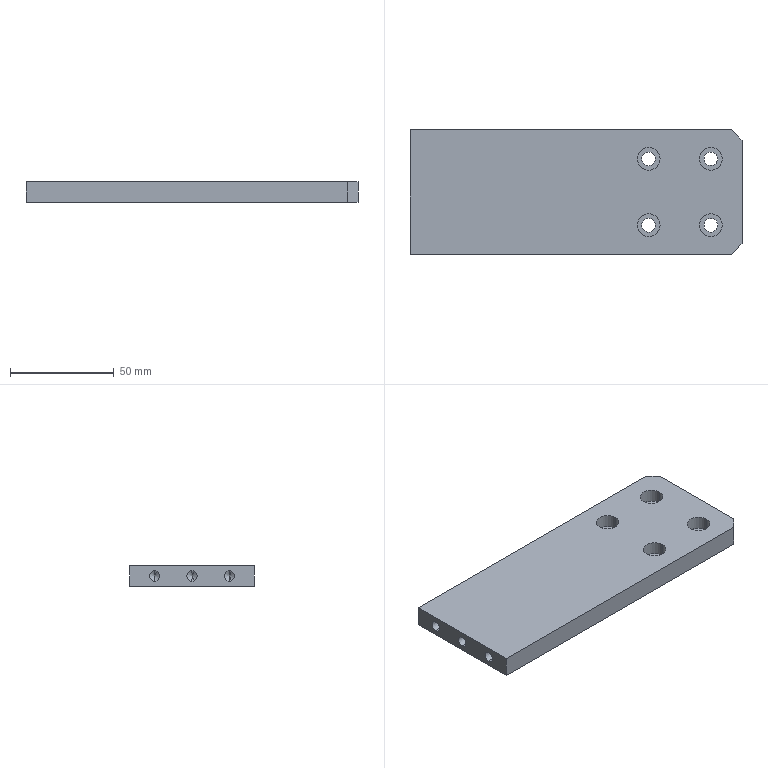Part | SolidWorks | features HoleWzd 2, Chamfer 1, Extrusion 1 | 1 solid | 40 faces | box 160 x 60 x 10 mm | volume 92147 mm3 | cylinder 22 | plane 12 | cone 6 | commonest cylinder face diameters 6.6 x8 11 x8 5 x6
STEP:
#1=CARTESIAN_POINT('',(-69.,18.,-2.5));
#2=VERTEX_POINT('',#1);
#3=CARTESIAN_POINT('',(-69.,18.,2.5));
#4=VERTEX_POINT('',#3);
#5=CARTESIAN_POINT('',(-69.,18.,0.));
#6=DIRECTION('',(-1.,0.,0.));
#7=DIRECTION('',(0.,0.,1.));
#8=AXIS2_PLACEMENT_3D('',#5,#6,#7);
#9=CIRCLE('',#8,2.5);
#10=EDGE_CURVE('',#2,#4,#9,.T.);
#11=ORIENTED_EDGE('',*,*,#10,.F.);
#12=CARTESIAN_POINT('',(-80.,18.,-2.5));
#13=VERTEX_POINT('',#12);
#14=CARTESIAN_POINT('',(-80.,18.,-2.5));
#15=DIRECTION('',(-1.,0.,0.));
#16=VECTOR('',#15,1000.);
#17=LINE('',#14,#16);
#18=EDGE_CURVE('',#2,#13,#17,.T.);
#19=ORIENTED_EDGE('',*,*,#18,.T.);
#20=CARTESIAN_POINT('',(-80.,18.,2.5));
#21=VERTEX_POINT('',#20);
#22=CARTESIAN_POINT('',(-80.,18.,0.));
#23=DIRECTION('',(-1.,0.,0.));
#24=DIRECTION('',(0.,0.,1.));
#25=AXIS2_PLACEMENT_3D('',#22,#23,#24);
#26=CIRCLE('',#25,2.5);
#27=EDGE_CURVE('',#13,#21,#26,.T.);
#28=ORIENTED_EDGE('',*,*,#27,.T.);
#29=CARTESIAN_POINT('',(-80.,18.,2.5));
#30=DIRECTION('',(-1.,0.,0.));
#31=VECTOR('',#30,1000.);
#32=LINE('',#29,#31);
#33=EDGE_CURVE('',#4,#21,#32,.T.);
#34=ORIENTED_EDGE('',*,*,#33,.F.);
#35=EDGE_LOOP('',(#11,#19,#28,#34));
#36=FACE_OUTER_BOUND('',#35,.T.);
#37=CARTESIAN_POINT('',(-80.,18.,0.));
#38=DIRECTION('',(-1.,0.,0.));
#39=DIRECTION('',(0.,0.,1.));
#40=AXIS2_PLACEMENT_3D('',#37,#38,#39);
#41=CYLINDRICAL_SURFACE('',#40,2.5);
#42=ADVANCED_FACE('',(#36),#41,.F.);
#43=CARTESIAN_POINT('',(-67.498,18.,0.));
#44=VERTEX_POINT('',#43);
#45=CARTESIAN_POINT('',(-69.,18.,2.5));
#46=DIRECTION('',(-0.515,0.,0.8572));
#47=VECTOR('',#46,1000.);
#48=LINE('',#45,#47);
#49=EDGE_CURVE('',#44,#4,#48,.T.);
#50=ORIENTED_EDGE('',*,*,#49,.F.);
#51=CARTESIAN_POINT('',(-69.,18.,-2.5));
#52=DIRECTION('',(-0.515,0.,-0.8572));
#53=VECTOR('',#52,1000.);
#54=LINE('',#51,#53);
#55=EDGE_CURVE('',#44,#2,#54,.T.);
#56=ORIENTED_EDGE('',*,*,#55,.T.);
#57=ORIENTED_EDGE('',*,*,#10,.T.);
#58=EDGE_LOOP('',(#50,#56,#57));
#59=FACE_OUTER_BOUND('',#58,.T.);
#60=CARTESIAN_POINT('',(-69.,18.,0.));
#61=DIRECTION('',(-1.,0.,0.));
#62=DIRECTION('',(0.,0.,1.));
#63=AXIS2_PLACEMENT_3D('',#60,#61,#62);
#64=CONICAL_SURFACE('',#63,2.5,1.03);
#65=ADVANCED_FACE('',(#59),#64,.F.);
#66=CARTESIAN_POINT('',(-69.,0.,-2.5));
#67=VERTEX_POINT('',#66);
#68=CARTESIAN_POINT('',(-69.,0.,2.5));
#69=VERTEX_POINT('',#68);
#70=CARTESIAN_POINT('',(-69.,0.,0.));
#71=DIRECTION('',(-1.,0.,0.));
#72=DIRECTION('',(0.,0.,1.));
#73=AXIS2_PLACEMENT_3D('',#70,#71,#72);
#74=CIRCLE('',#73,2.5);
#75=EDGE_CURVE('',#67,#69,#74,.T.);
#76=ORIENTED_EDGE('',*,*,#75,.F.);
#77=CARTESIAN_POINT('',(-80.,0.,-2.5));
#78=VERTEX_POINT('',#77);
#79=CARTESIAN_POINT('',(-80.,0.,-2.5));
#80=DIRECTION('',(-1.,0.,0.));
#81=VECTOR('',#80,1000.);
#82=LINE('',#79,#81);
#83=EDGE_CURVE('',#67,#78,#82,.T.);
#84=ORIENTED_EDGE('',*,*,#83,.T.);
#85=CARTESIAN_POINT('',(-80.,0.,2.5));
#86=VERTEX_POINT('',#85);
#87=CARTESIAN_POINT('',(-80.,0.,0.));
#88=DIRECTION('',(-1.,0.,0.));
#89=DIRECTION('',(0.,0.,1.));
#90=AXIS2_PLACEMENT_3D('',#87,#88,#89);
#91=CIRCLE('',#90,2.5);
#92=EDGE_CURVE('',#78,#86,#91,.T.);
#93=ORIENTED_EDGE('',*,*,#92,.T.);
#94=CARTESIAN_POINT('',(-80.,0.,2.5));
#95=DIRECTION('',(-1.,0.,0.));
#96=VECTOR('',#95,1000.);
#97=LINE('',#94,#96);
#98=EDGE_CURVE('',#69,#86,#97,.T.);
#99=ORIENTED_EDGE('',*,*,#98,.F.);
#100=EDGE_LOOP('',(#76,#84,#93,#99));
#101=FACE_OUTER_BOUND('',#100,.T.);
#102=CARTESIAN_POINT('',(-80.,0.,0.));
#103=DIRECTION('',(-1.,0.,0.));
#104=DIRECTION('',(0.,0.,1.));
#105=AXIS2_PLACEMENT_3D('',#102,#103,#104);
#106=CYLINDRICAL_SURFACE('',#105,2.5);
#107=ADVANCED_FACE('',(#101),#106,.F.);
#108=CARTESIAN_POINT('',(-67.498,0.,0.));
#109=VERTEX_POINT('',#108);
#110=CARTESIAN_POINT('',(-69.,0.,2.5));
#111=DIRECTION('',(-0.515,0.,0.8572));
#112=VECTOR('',#111,1000.);
#113=LINE('',#110,#112);
#114=EDGE_CURVE('',#109,#69,#113,.T.);
#115=ORIENTED_EDGE('',*,*,#114,.F.);
#116=CARTESIAN_POINT('',(-69.,0.,-2.5));
#117=DIRECTION('',(-0.515,0.,-0.8572));
#118=VECTOR('',#117,1000.);
#119=LINE('',#116,#118);
#120=EDGE_CURVE('',#109,#67,#119,.T.);
#121=ORIENTED_EDGE('',*,*,#120,.T.);
#122=ORIENTED_EDGE('',*,*,#75,.T.);
#123=EDGE_LOOP('',(#115,#121,#122));
#124=FACE_OUTER_BOUND('',#123,.T.);
#125=CARTESIAN_POINT('',(-69.,0.,0.));
#126=DIRECTION('',(-1.,0.,0.));
#127=DIRECTION('',(0.,0.,1.));
#128=AXIS2_PLACEMENT_3D('',#125,#126,#127);
#129=CONICAL_SURFACE('',#128,2.5,1.03);
#130=ADVANCED_FACE('',(#124),#129,.F.);
#131=CARTESIAN_POINT('',(-69.,-18.,-2.5));
#132=VERTEX_POINT('',#131);
#133=CARTESIAN_POINT('',(-69.,-18.,2.5));
#134=VERTEX_POINT('',#133);
#135=CARTESIAN_POINT('',(-69.,-18.,0.));
#136=DIRECTION('',(-1.,0.,0.));
#137=DIRECTION('',(0.,0.,1.));
#138=AXIS2_PLACEMENT_3D('',#135,#136,#137);
#139=CIRCLE('',#138,2.5);
#140=EDGE_CURVE('',#132,#134,#139,.T.);
#141=ORIENTED_EDGE('',*,*,#140,.F.);
#142=CARTESIAN_POINT('',(-80.,-18.,-2.5));
#143=VERTEX_POINT('',#142);
#144=CARTESIAN_POINT('',(-80.,-18.,-2.5));
#145=DIRECTION('',(-1.,0.,0.));
#146=VECTOR('',#145,1000.);
#147=LINE('',#144,#146);
#148=EDGE_CURVE('',#132,#143,#147,.T.);
#149=ORIENTED_EDGE('',*,*,#148,.T.);
#150=CARTESIAN_POINT('',(-80.,-18.,2.5));
#151=VERTEX_POINT('',#150);
#152=CARTESIAN_POINT('',(-80.,-18.,0.));
#153=DIRECTION('',(-1.,0.,0.));
#154=DIRECTION('',(0.,0.,1.));
#155=AXIS2_PLACEMENT_3D('',#152,#153,#154);
#156=CIRCLE('',#155,2.5);
#157=EDGE_CURVE('',#143,#151,#156,.T.);
#158=ORIENTED_EDGE('',*,*,#157,.T.);
#159=CARTESIAN_POINT('',(-80.,-18.,2.5));
#160=DIRECTION('',(-1.,0.,0.));
#161=VECTOR('',#160,1000.);
#162=LINE('',#159,#161);
#163=EDGE_CURVE('',#134,#151,#162,.T.);
#164=ORIENTED_EDGE('',*,*,#163,.F.);
#165=EDGE_LOOP('',(#141,#149,#158,#164));
#166=FACE_OUTER_BOUND('',#165,.T.);
#167=CARTESIAN_POINT('',(-80.,-18.,0.));
#168=DIRECTION('',(-1.,0.,0.));
#169=DIRECTION('',(0.,0.,1.));
#170=AXIS2_PLACEMENT_3D('',#167,#168,#169);
#171=CYLINDRICAL_SURFACE('',#170,2.5);
#172=ADVANCED_FACE('',(#166),#171,.F.);
#173=CARTESIAN_POINT('',(-67.498,-18.,0.));
#174=VERTEX_POINT('',#173);
#175=CARTESIAN_POINT('',(-69.,-18.,2.5));
#176=DIRECTION('',(-0.515,0.,0.8572));
#177=VECTOR('',#176,1000.);
#178=LINE('',#175,#177);
#179=EDGE_CURVE('',#174,#134,#178,.T.);
#180=ORIENTED_EDGE('',*,*,#179,.F.);
#181=CARTESIAN_POINT('',(-69.,-18.,-2.5));
#182=DIRECTION('',(-0.515,0.,-0.8572));
#183=VECTOR('',#182,1000.);
#184=LINE('',#181,#183);
#185=EDGE_CURVE('',#174,#132,#184,.T.);
#186=ORIENTED_EDGE('',*,*,#185,.T.);
#187=ORIENTED_EDGE('',*,*,#140,.T.);
#188=EDGE_LOOP('',(#180,#186,#187));
#189=FACE_OUTER_BOUND('',#188,.T.);
#190=CARTESIAN_POINT('',(-69.,-18.,0.));
#191=DIRECTION('',(-1.,0.,0.));
#192=DIRECTION('',(0.,0.,1.));
#193=AXIS2_PLACEMENT_3D('',#190,#191,#192);
#194=CONICAL_SURFACE('',#193,2.5,1.03);
#195=ADVANCED_FACE('',(#189),#194,.F.);
#196=CARTESIAN_POINT('',(29.5,-16.,-1.4));
#197=VERTEX_POINT('',#196);
#198=CARTESIAN_POINT('',(40.5,-16.,-1.4));
#199=VERTEX_POINT('',#198);
#200=CARTESIAN_POINT('',(35.,-16.,-1.4));
#201=DIRECTION('',(0.,0.,1.));
#202=DIRECTION('',(1.,0.,0.));
#203=AXIS2_PLACEMENT_3D('',#200,#201,#202);
#204=CIRCLE('',#203,5.5);
#205=EDGE_CURVE('',#197,#199,#204,.T.);
#206=ORIENTED_EDGE('',*,*,#205,.F.);
#207=CARTESIAN_POINT('',(29.5,-16.,5.));
#208=VERTEX_POINT('',#207);
#209=CARTESIAN_POINT('',(29.5,-16.,5.));
#210=DIRECTION('',(0.,0.,1.));
#211=VECTOR('',#210,1000.);
#212=LINE('',#209,#211);
#213=EDGE_CURVE('',#197,#208,#212,.T.);
#214=ORIENTED_EDGE('',*,*,#213,.T.);
#215=CARTESIAN_POINT('',(40.5,-16.,5.));
#216=VERTEX_POINT('',#215);
#217=CARTESIAN_POINT('',(35.,-16.,5.));
#218=DIRECTION('',(0.,0.,1.));
#219=DIRECTION('',(1.,0.,0.));
#220=AXIS2_PLACEMENT_3D('',#217,#218,#219);
#221=CIRCLE('',#220,5.5);
#222=EDGE_CURVE('',#208,#216,#221,.T.);
#223=ORIENTED_EDGE('',*,*,#222,.T.);
#224=CARTESIAN_POINT('',(40.5,-16.,5.));
#225=DIRECTION('',(0.,0.,1.));
#226=VECTOR('',#225,1000.);
#227=LINE('',#224,#226);
#228=EDGE_CURVE('',#199,#216,#227,.T.);
#229=ORIENTED_EDGE('',*,*,#228,.F.);
#230=EDGE_LOOP('',(#206,#214,#223,#229));
#231=FACE_OUTER_BOUND('',#230,.T.);
#232=CARTESIAN_POINT('',(35.,-16.,5.));
#233=DIRECTION('',(0.,0.,1.));
#234=DIRECTION('',(1.,0.,0.));
#235=AXIS2_PLACEMENT_3D('',#232,#233,#234);
#236=CYLINDRICAL_SURFACE('',#235,5.5);
#237=ADVANCED_FACE('',(#231),#236,.F.);
#238=CARTESIAN_POINT('',(31.7,-16.,-5.));
#239=VERTEX_POINT('',#238);
#240=CARTESIAN_POINT('',(38.3,-16.,-5.));
#241=VERTEX_POINT('',#240);
#242=CARTESIAN_POINT('',(35.,-16.,-5.));
#243=DIRECTION('',(0.,0.,1.));
#244=DIRECTION('',(1.,0.,0.));
#245=AXIS2_PLACEMENT_3D('',#242,#243,#244);
#246=CIRCLE('',#245,3.3);
#247=EDGE_CURVE('',#239,#241,#246,.T.);
#248=ORIENTED_EDGE('',*,*,#247,.F.);
#249=CARTESIAN_POINT('',(31.7,-16.,-1.4));
#250=VERTEX_POINT('',#249);
#251=CARTESIAN_POINT('',(31.7,-16.,5.));
#252=DIRECTION('',(0.,0.,1.));
#253=VECTOR('',#252,1000.);
#254=LINE('',#251,#253);
#255=EDGE_CURVE('',#239,#250,#254,.T.);
#256=ORIENTED_EDGE('',*,*,#255,.T.);
#257=CARTESIAN_POINT('',(38.3,-16.,-1.4));
#258=VERTEX_POINT('',#257);
#259=CARTESIAN_POINT('',(35.,-16.,-1.4));
#260=DIRECTION('',(0.,0.,1.));
#261=DIRECTION('',(1.,0.,0.));
#262=AXIS2_PLACEMENT_3D('',#259,#260,#261);
#263=CIRCLE('',#262,3.3);
#264=EDGE_CURVE('',#250,#258,#263,.T.);
#265=ORIENTED_EDGE('',*,*,#264,.T.);
#266=CARTESIAN_POINT('',(38.3,-16.,5.));
#267=DIRECTION('',(0.,0.,1.));
#268=VECTOR('',#267,1000.);
#269=LINE('',#266,#268);
#270=EDGE_CURVE('',#241,#258,#269,.T.);
#271=ORIENTED_EDGE('',*,*,#270,.F.);
#272=EDGE_LOOP('',(#248,#256,#265,#271));
#273=FACE_OUTER_BOUND('',#272,.T.);
#274=CARTESIAN_POINT('',(35.,-16.,5.));
#275=DIRECTION('',(0.,0.,1.));
#276=DIRECTION('',(1.,0.,0.));
#277=AXIS2_PLACEMENT_3D('',#274,#275,#276);
#278=CYLINDRICAL_SURFACE('',#277,3.3);
#279=ADVANCED_FACE('',(#273),#278,.F.);
#280=CARTESIAN_POINT('',(59.5,-16.,-1.4));
#281=VERTEX_POINT('',#280);
#282=CARTESIAN_POINT('',(70.5,-16.,-1.4));
#283=VERTEX_POINT('',#282);
#284=CARTESIAN_POINT('',(65.,-16.,-1.4));
#285=DIRECTION('',(0.,0.,1.));
#286=DIRECTION('',(1.,0.,0.));
#287=AXIS2_PLACEMENT_3D('',#284,#285,#286);
#288=CIRCLE('',#287,5.5);
#289=EDGE_CURVE('',#281,#283,#288,.T.);
#290=ORIENTED_EDGE('',*,*,#289,.F.);
#291=CARTESIAN_POINT('',(59.5,-16.,5.));
#292=VERTEX_POINT('',#291);
#293=CARTESIAN_POINT('',(59.5,-16.,5.));
#294=DIRECTION('',(0.,0.,1.));
#295=VECTOR('',#294,1000.);
#296=LINE('',#293,#295);
#297=EDGE_CURVE('',#281,#292,#296,.T.);
#298=ORIENTED_EDGE('',*,*,#297,.T.);
#299=CARTESIAN_POINT('',(70.5,-16.,5.));
#300=VERTEX_POINT('',#299);
#301=CARTESIAN_POINT('',(65.,-16.,5.));
#302=DIRECTION('',(0.,0.,1.));
#303=DIRECTION('',(1.,0.,0.));
#304=AXIS2_PLACEMENT_3D('',#301,#302,#303);
#305=CIRCLE('',#304,5.5);
#306=EDGE_CURVE('',#292,#300,#305,.T.);
#307=ORIENTED_EDGE('',*,*,#306,.T.);
#308=CARTESIAN_POINT('',(70.5,-16.,5.));
#309=DIRECTION('',(0.,0.,1.));
#310=VECTOR('',#309,1000.);
#311=LINE('',#308,#310);
#312=EDGE_CURVE('',#283,#300,#311,.T.);
#313=ORIENTED_EDGE('',*,*,#312,.F.);
#314=EDGE_LOOP('',(#290,#298,#307,#313));
#315=FACE_OUTER_BOUND('',#314,.T.);
#316=CARTESIAN_POINT('',(65.,-16.,5.));
#317=DIRECTION('',(0.,0.,1.));
#318=DIRECTION('',(1.,0.,0.));
#319=AXIS2_PLACEMENT_3D('',#316,#317,#318);
#320=CYLINDRICAL_SURFACE('',#319,5.5);
#321=ADVANCED_FACE('',(#315),#320,.F.);
#322=CARTESIAN_POINT('',(61.7,-16.,-5.));
#323=VERTEX_POINT('',#322);
#324=CARTESIAN_POINT('',(68.3,-16.,-5.));
#325=VERTEX_POINT('',#324);
#326=CARTESIAN_POINT('',(65.,-16.,-5.));
#327=DIRECTION('',(0.,0.,1.));
#328=DIRECTION('',(1.,0.,0.));
#329=AXIS2_PLACEMENT_3D('',#326,#327,#328);
#330=CIRCLE('',#329,3.3);
#331=EDGE_CURVE('',#323,#325,#330,.T.);
#332=ORIENTED_EDGE('',*,*,#331,.F.);
#333=CARTESIAN_POINT('',(61.7,-16.,-1.4));
#334=VERTEX_POINT('',#333);
#335=CARTESIAN_POINT('',(61.7,-16.,5.));
#336=DIRECTION('',(0.,0.,1.));
#337=VECTOR('',#336,1000.);
#338=LINE('',#335,#337);
#339=EDGE_CURVE('',#323,#334,#338,.T.);
#340=ORIENTED_EDGE('',*,*,#339,.T.);
#341=CARTESIAN_POINT('',(68.3,-16.,-1.4));
#342=VERTEX_POINT('',#341);
#343=CARTESIAN_POINT('',(65.,-16.,-1.4));
#344=DIRECTION('',(0.,0.,1.));
#345=DIRECTION('',(1.,0.,0.));
#346=AXIS2_PLACEMENT_3D('',#343,#344,#345);
#347=CIRCLE('',#346,3.3);
#348=EDGE_CURVE('',#334,#342,#347,.T.);
#349=ORIENTED_EDGE('',*,*,#348,.T.);
#350=CARTESIAN_POINT('',(68.3,-16.,5.));
#351=DIRECTION('',(0.,0.,1.));
#352=VECTOR('',#351,1000.);
#353=LINE('',#350,#352);
#354=EDGE_CURVE('',#325,#342,#353,.T.);
#355=ORIENTED_EDGE('',*,*,#354,.F.);
#356=EDGE_LOOP('',(#332,#340,#349,#355));
#357=FACE_OUTER_BOUND('',#356,.T.);
#358=CARTESIAN_POINT('',(65.,-16.,5.));
#359=DIRECTION('',(0.,0.,1.));
#360=DIRECTION('',(1.,0.,0.));
#361=AXIS2_PLACEMENT_3D('',#358,#359,#360);
#362=CYLINDRICAL_SURFACE('',#361,3.3);
#363=ADVANCED_FACE('',(#357),#362,.F.);
#364=CARTESIAN_POINT('',(59.5,16.,-1.4));
#365=VERTEX_POINT('',#364);
#366=CARTESIAN_POINT('',(70.5,16.,-1.4));
#367=VERTEX_POINT('',#366);
#368=CARTESIAN_POINT('',(65.,16.,-1.4));
#369=DIRECTION('',(0.,0.,1.));
#370=DIRECTION('',(1.,0.,0.));
#371=AXIS2_PLACEMENT_3D('',#368,#369,#370);
#372=CIRCLE('',#371,5.5);
#373=EDGE_CURVE('',#365,#367,#372,.T.);
#374=ORIENTED_EDGE('',*,*,#373,.F.);
#375=CARTESIAN_POINT('',(59.5,16.,5.));
#376=VERTEX_POINT('',#375);
#377=CARTESIAN_POINT('',(59.5,16.,5.));
#378=DIRECTION('',(0.,0.,1.));
#379=VECTOR('',#378,1000.);
#380=LINE('',#377,#379);
#381=EDGE_CURVE('',#365,#376,#380,.T.);
#382=ORIENTED_EDGE('',*,*,#381,.T.);
#383=CARTESIAN_POINT('',(70.5,16.,5.));
#384=VERTEX_POINT('',#383);
#385=CARTESIAN_POINT('',(65.,16.,5.));
#386=DIRECTION('',(0.,0.,1.));
#387=DIRECTION('',(1.,0.,0.));
#388=AXIS2_PLACEMENT_3D('',#385,#386,#387);
#389=CIRCLE('',#388,5.5);
#390=EDGE_CURVE('',#376,#384,#389,.T.);
#391=ORIENTED_EDGE('',*,*,#390,.T.);
#392=CARTESIAN_POINT('',(70.5,16.,5.));
#393=DIRECTION('',(0.,0.,1.));
#394=VECTOR('',#393,1000.);
#395=LINE('',#392,#394);
#396=EDGE_CURVE('',#367,#384,#395,.T.);
#397=ORIENTED_EDGE('',*,*,#396,.F.);
#398=EDGE_LOOP('',(#374,#382,#391,#397));
#399=FACE_OUTER_BOUND('',#398,.T.);
#400=CARTESIAN_POINT('',(65.,16.,5.));
#401=DIRECTION('',(0.,0.,1.));
#402=DIRECTION('',(1.,0.,0.));
#403=AXIS2_PLACEMENT_3D('',#400,#401,#402);
#404=CYLINDRICAL_SURFACE('',#403,5.5);
#405=ADVANCED_FACE('',(#399),#404,.F.);
#406=CARTESIAN_POINT('',(61.7,16.,-5.));
#407=VERTEX_POINT('',#406);
#408=CARTESIAN_POINT('',(68.3,16.,-5.));
#409=VERTEX_POINT('',#408);
#410=CARTESIAN_POINT('',(65.,16.,-5.));
#411=DIRECTION('',(0.,0.,1.));
#412=DIRECTION('',(1.,0.,0.));
#413=AXIS2_PLACEMENT_3D('',#410,#411,#412);
#414=CIRCLE('',#413,3.3);
#415=EDGE_CURVE('',#407,#409,#414,.T.);
#416=ORIENTED_EDGE('',*,*,#415,.F.);
#417=CARTESIAN_POINT('',(61.7,16.,-1.4));
#418=VERTEX_POINT('',#417);
#419=CARTESIAN_POINT('',(61.7,16.,5.));
#420=DIRECTION('',(0.,0.,1.));
#421=VECTOR('',#420,1000.);
#422=LINE('',#419,#421);
#423=EDGE_CURVE('',#407,#418,#422,.T.);
#424=ORIENTED_EDGE('',*,*,#423,.T.);
#425=CARTESIAN_POINT('',(68.3,16.,-1.4));
#426=VERTEX_POINT('',#425);
#427=CARTESIAN_POINT('',(65.,16.,-1.4));
#428=DIRECTION('',(0.,0.,1.));
#429=DIRECTION('',(1.,0.,0.));
#430=AXIS2_PLACEMENT_3D('',#427,#428,#429);
#431=CIRCLE('',#430,3.3);
#432=EDGE_CURVE('',#418,#426,#431,.T.);
#433=ORIENTED_EDGE('',*,*,#432,.T.);
#434=CARTESIAN_POINT('',(68.3,16.,5.));
#435=DIRECTION('',(0.,0.,1.));
#436=VECTOR('',#435,1000.);
#437=LINE('',#434,#436);
#438=EDGE_CURVE('',#409,#426,#437,.T.);
#439=ORIENTED_EDGE('',*,*,#438,.F.);
#440=EDGE_LOOP('',(#416,#424,#433,#439));
#441=FACE_OUTER_BOUND('',#440,.T.);
#442=CARTESIAN_POINT('',(65.,16.,5.));
#443=DIRECTION('',(0.,0.,1.));
#444=DIRECTION('',(1.,0.,0.));
#445=AXIS2_PLACEMENT_3D('',#442,#443,#444);
#446=CYLINDRICAL_SURFACE('',#445,3.3);
#447=ADVANCED_FACE('',(#441),#446,.F.);
#448=CARTESIAN_POINT('',(29.5,16.,-1.4));
#449=VERTEX_POINT('',#448);
#450=CARTESIAN_POINT('',(40.5,16.,-1.4));
#451=VERTEX_POINT('',#450);
#452=CARTESIAN_POINT('',(35.,16.,-1.4));
#453=DIRECTION('',(0.,0.,1.));
#454=DIRECTION('',(1.,0.,0.));
#455=AXIS2_PLACEMENT_3D('',#452,#453,#454);
#456=CIRCLE('',#455,5.5);
#457=EDGE_CURVE('',#449,#451,#456,.T.);
#458=ORIENTED_EDGE('',*,*,#457,.F.);
#459=CARTESIAN_POINT('',(29.5,16.,5.));
#460=VERTEX_POINT('',#459);
#461=CARTESIAN_POINT('',(29.5,16.,5.));
#462=DIRECTION('',(0.,0.,1.));
#463=VECTOR('',#462,1000.);
#464=LINE('',#461,#463);
#465=EDGE_CURVE('',#449,#460,#464,.T.);
#466=ORIENTED_EDGE('',*,*,#465,.T.);
#467=CARTESIAN_POINT('',(40.5,16.,5.));
#468=VERTEX_POINT('',#467);
#469=CARTESIAN_POINT('',(35.,16.,5.));
#470=DIRECTION('',(0.,0.,1.));
#471=DIRECTION('',(1.,0.,0.));
#472=AXIS2_PLACEMENT_3D('',#469,#470,#471);
#473=CIRCLE('',#472,5.5);
#474=EDGE_CURVE('',#460,#468,#473,.T.);
#475=ORIENTED_EDGE('',*,*,#474,.T.);
#476=CARTESIAN_POINT('',(40.5,16.,5.));
#477=DIRECTION('',(0.,0.,1.));
#478=VECTOR('',#477,1000.);
#479=LINE('',#476,#478);
#480=EDGE_CURVE('',#451,#468,#479,.T.);
#481=ORIENTED_EDGE('',*,*,#480,.F.);
#482=EDGE_LOOP('',(#458,#466,#475,#481));
#483=FACE_OUTER_BOUND('',#482,.T.);
#484=CARTESIAN_POINT('',(35.,16.,5.));
#485=DIRECTION('',(0.,0.,1.));
#486=DIRECTION('',(1.,0.,0.));
#487=AXIS2_PLACEMENT_3D('',#484,#485,#486);
#488=CYLINDRICAL_SURFACE('',#487,5.5);
#489=ADVANCED_FACE('',(#483),#488,.F.);
#490=CARTESIAN_POINT('',(31.7,16.,-5.));
#491=VERTEX_POINT('',#490);
#492=CARTESIAN_POINT('',(38.3,16.,-5.));
#493=VERTEX_POINT('',#492);
#494=CARTESIAN_POINT('',(35.,16.,-5.));
#495=DIRECTION('',(0.,0.,1.));
#496=DIRECTION('',(1.,0.,0.));
#497=AXIS2_PLACEMENT_3D('',#494,#495,#496);
#498=CIRCLE('',#497,3.3);
#499=EDGE_CURVE('',#491,#493,#498,.T.);
#500=ORIENTED_EDGE('',*,*,#499,.F.);
#501=CARTESIAN_POINT('',(31.7,16.,-1.4));
#502=VERTEX_POINT('',#501);
#503=CARTESIAN_POINT('',(31.7,16.,5.));
#504=DIRECTION('',(0.,0.,1.));
#505=VECTOR('',#504,1000.);
#506=LINE('',#503,#505);
#507=EDGE_CURVE('',#491,#502,#506,.T.);
#508=ORIENTED_EDGE('',*,*,#507,.T.);
#509=CARTESIAN_POINT('',(38.3,16.,-1.4));
#510=VERTEX_POINT('',#509);
#511=CARTESIAN_POINT('',(35.,16.,-1.4));
#512=DIRECTION('',(0.,0.,1.));
#513=DIRECTION('',(1.,0.,0.));
#514=AXIS2_PLACEMENT_3D('',#511,#512,#513);
#515=CIRCLE('',#514,3.3);
#516=EDGE_CURVE('',#502,#510,#515,.T.);
#517=ORIENTED_EDGE('',*,*,#516,.T.);
#518=CARTESIAN_POINT('',(38.3,16.,5.));
#519=DIRECTION('',(0.,0.,1.));
#520=VECTOR('',#519,1000.);
#521=LINE('',#518,#520);
#522=EDGE_CURVE('',#493,#510,#521,.T.);
#523=ORIENTED_EDGE('',*,*,#522,.F.);
#524=EDGE_LOOP('',(#500,#508,#517,#523));
#525=FACE_OUTER_BOUND('',#524,.T.);
#526=CARTESIAN_POINT('',(35.,16.,5.));
#527=DIRECTION('',(0.,0.,1.));
#528=DIRECTION('',(1.,0.,0.));
#529=AXIS2_PLACEMENT_3D('',#526,#527,#528);
#530=CYLINDRICAL_SURFACE('',#529,3.3);
#531=ADVANCED_FACE('',(#525),#530,.F.);
#532=CARTESIAN_POINT('',(80.,-25.,-5.));
#533=VERTEX_POINT('',#532);
#534=CARTESIAN_POINT('',(80.,25.,-5.));
#535=VERTEX_POINT('',#534);
#536=CARTESIAN_POINT('',(80.,-30.,-5.));
#537=DIRECTION('',(0.,1.,0.));
#538=VECTOR('',#537,1000.);
#539=LINE('',#536,#538);
#540=EDGE_CURVE('',#533,#535,#539,.T.);
#541=ORIENTED_EDGE('',*,*,#540,.T.);
#542=CARTESIAN_POINT('',(80.,25.,5.));
#543=VERTEX_POINT('',#542);
#544=CARTESIAN_POINT('',(80.,25.,5.));
#545=DIRECTION('',(0.,0.,1.));
#546=VECTOR('',#545,1000.);
#547=LINE('',#544,#546);
#548=EDGE_CURVE('',#535,#543,#547,.T.);
#549=ORIENTED_EDGE('',*,*,#548,.T.);
#550=CARTESIAN_POINT('',(80.,-25.,5.));
#551=VERTEX_POINT('',#550);
#552=CARTESIAN_POINT('',(80.,-30.,5.));
#553=DIRECTION('',(0.,1.,0.));
#554=VECTOR('',#553,1000.);
#555=LINE('',#552,#554);
#556=EDGE_CURVE('',#551,#543,#555,.T.);
#557=ORIENTED_EDGE('',*,*,#556,.F.);
#558=CARTESIAN_POINT('',(80.,-25.,5.));
#559=DIRECTION('',(0.,0.,-1.));
#560=VECTOR('',#559,1000.);
#561=LINE('',#558,#560);
#562=EDGE_CURVE('',#551,#533,#561,.T.);
#563=ORIENTED_EDGE('',*,*,#562,.T.);
#564=EDGE_LOOP('',(#541,#549,#557,#563));
#565=FACE_OUTER_BOUND('',#564,.T.);
#566=CARTESIAN_POINT('',(80.,-30.,5.));
#567=DIRECTION('',(-1.,0.,0.));
#568=DIRECTION('',(0.,0.,1.));
#569=AXIS2_PLACEMENT_3D('',#566,#567,#568);
#570=PLANE('',#569);
#571=ADVANCED_FACE('',(#565),#570,.F.);
#572=CARTESIAN_POINT('',(75.,30.,5.));
#573=VERTEX_POINT('',#572);
#574=CARTESIAN_POINT('',(-80.,30.,5.));
#575=VERTEX_POINT('',#574);
#576=CARTESIAN_POINT('',(-80.,30.,5.));
#577=DIRECTION('',(-1.,0.,0.));
#578=VECTOR('',#577,1000.);
#579=LINE('',#576,#578);
#580=EDGE_CURVE('',#573,#575,#579,.T.);
#581=ORIENTED_EDGE('',*,*,#580,.F.);
#582=CARTESIAN_POINT('',(75.,30.,-5.));
#583=VERTEX_POINT('',#582);
#584=CARTESIAN_POINT('',(75.,30.,5.));
#585=DIRECTION('',(0.,0.,-1.));
#586=VECTOR('',#585,1000.);
#587=LINE('',#584,#586);
#588=EDGE_CURVE('',#573,#583,#587,.T.);
#589=ORIENTED_EDGE('',*,*,#588,.T.);
#590=CARTESIAN_POINT('',(-80.,30.,-5.));
#591=VERTEX_POINT('',#590);
#592=CARTESIAN_POINT('',(-80.,30.,-5.));
#593=DIRECTION('',(-1.,0.,0.));
#594=VECTOR('',#593,1000.);
#595=LINE('',#592,#594);
#596=EDGE_CURVE('',#583,#591,#595,.T.);
#597=ORIENTED_EDGE('',*,*,#596,.T.);
#598=CARTESIAN_POINT('',(-80.,30.,5.));
#599=DIRECTION('',(0.,0.,-1.));
#600=VECTOR('',#599,1000.);
#601=LINE('',#598,#600);
#602=EDGE_CURVE('',#575,#591,#601,.T.);
#603=ORIENTED_EDGE('',*,*,#602,.F.);
#604=EDGE_LOOP('',(#581,#589,#597,#603));
#605=FACE_OUTER_BOUND('',#604,.T.);
#606=CARTESIAN_POINT('',(-80.,30.,5.));
#607=DIRECTION('',(0.,-1.,0.));
#608=DIRECTION('',(0.,0.,-1.));
#609=AXIS2_PLACEMENT_3D('',#606,#607,#608);
#610=PLANE('',#609);
#611=ADVANCED_FACE('',(#605),#610,.F.);
#612=CARTESIAN_POINT('',(-80.,18.,0.));
#613=DIRECTION('',(-1.,0.,0.));
#614=DIRECTION('',(0.,0.,1.));
#615=AXIS2_PLACEMENT_3D('',#612,#613,#614);
#616=CIRCLE('',#615,2.5);
#617=EDGE_CURVE('',#21,#13,#616,.T.);
#618=ORIENTED_EDGE('',*,*,#617,.F.);
#619=ORIENTED_EDGE('',*,*,#27,.F.);
#620=EDGE_LOOP('',(#618,#619));
#621=FACE_BOUND('',#620,.T.);
#622=CARTESIAN_POINT('',(-80.,0.,0.));
#623=DIRECTION('',(-1.,0.,0.));
#624=DIRECTION('',(0.,0.,1.));
#625=AXIS2_PLACEMENT_3D('',#622,#623,#624);
#626=CIRCLE('',#625,2.5);
#627=EDGE_CURVE('',#86,#78,#626,.T.);
#628=ORIENTED_EDGE('',*,*,#627,.F.);
#629=ORIENTED_EDGE('',*,*,#92,.F.);
#630=EDGE_LOOP('',(#628,#629));
#631=FACE_BOUND('',#630,.T.);
#632=CARTESIAN_POINT('',(-80.,-18.,0.));
#633=DIRECTION('',(-1.,0.,0.));
#634=DIRECTION('',(0.,0.,1.));
#635=AXIS2_PLACEMENT_3D('',#632,#633,#634);
#636=CIRCLE('',#635,2.5);
#637=EDGE_CURVE('',#151,#143,#636,.T.);
#638=ORIENTED_EDGE('',*,*,#637,.F.);
#639=ORIENTED_EDGE('',*,*,#157,.F.);
#640=EDGE_LOOP('',(#638,#639));
#641=FACE_BOUND('',#640,.T.);
#642=CARTESIAN_POINT('',(-80.,-30.,-5.));
#643=VERTEX_POINT('',#642);
#644=CARTESIAN_POINT('',(-80.,-30.,-5.));
#645=DIRECTION('',(0.,-1.,0.));
#646=VECTOR('',#645,1000.);
#647=LINE('',#644,#646);
#648=EDGE_CURVE('',#591,#643,#647,.T.);
#649=ORIENTED_EDGE('',*,*,#648,.T.);
#650=CARTESIAN_POINT('',(-80.,-30.,5.));
#651=VERTEX_POINT('',#650);
#652=CARTESIAN_POINT('',(-80.,-30.,5.));
#653=DIRECTION('',(0.,0.,-1.));
#654=VECTOR('',#653,1000.);
#655=LINE('',#652,#654);
#656=EDGE_CURVE('',#651,#643,#655,.T.);
#657=ORIENTED_EDGE('',*,*,#656,.F.);
#658=CARTESIAN_POINT('',(-80.,-30.,5.));
#659=DIRECTION('',(0.,-1.,0.));
#660=VECTOR('',#659,1000.);
#661=LINE('',#658,#660);
#662=EDGE_CURVE('',#575,#651,#661,.T.);
#663=ORIENTED_EDGE('',*,*,#662,.F.);
#664=ORIENTED_EDGE('',*,*,#602,.T.);
#665=EDGE_LOOP('',(#649,#657,#663,#664));
#666=FACE_OUTER_BOUND('',#665,.T.);
#667=CARTESIAN_POINT('',(-80.,-30.,5.));
#668=DIRECTION('',(1.,0.,0.));
#669=DIRECTION('',(0.,0.,-1.));
#670=AXIS2_PLACEMENT_3D('',#667,#668,#669);
#671=PLANE('',#670);
#672=ADVANCED_FACE('',(#621,#631,#641,#666),#671,.F.);
#673=CARTESIAN_POINT('',(75.,-30.,-5.));
#674=VERTEX_POINT('',#673);
#675=CARTESIAN_POINT('',(-80.,-30.,-5.));
#676=DIRECTION('',(1.,0.,0.));
#677=VECTOR('',#676,1000.);
#678=LINE('',#675,#677);
#679=EDGE_CURVE('',#643,#674,#678,.T.);
#680=ORIENTED_EDGE('',*,*,#679,.T.);
#681=CARTESIAN_POINT('',(75.,-30.,5.));
#682=VERTEX_POINT('',#681);
#683=CARTESIAN_POINT('',(75.,-30.,5.));
#684=DIRECTION('',(0.,0.,1.));
#685=VECTOR('',#684,1000.);
#686=LINE('',#683,#685);
#687=EDGE_CURVE('',#674,#682,#686,.T.);
#688=ORIENTED_EDGE('',*,*,#687,.T.);
#689=CARTESIAN_POINT('',(-80.,-30.,5.));
#690=DIRECTION('',(1.,0.,0.));
#691=VECTOR('',#690,1000.);
#692=LINE('',#689,#691);
#693=EDGE_CURVE('',#651,#682,#692,.T.);
#694=ORIENTED_EDGE('',*,*,#693,.F.);
#695=ORIENTED_EDGE('',*,*,#656,.T.);
#696=EDGE_LOOP('',(#680,#688,#694,#695));
#697=FACE_OUTER_BOUND('',#696,.T.);
#698=CARTESIAN_POINT('',(-80.,-30.,5.));
#699=DIRECTION('',(0.,1.,0.));
#700=DIRECTION('',(0.,0.,1.));
#701=AXIS2_PLACEMENT_3D('',#698,#699,#700);
#702=PLANE('',#701);
#703=ADVANCED_FACE('',(#697),#702,.F.);
#704=CARTESIAN_POINT('',(35.,-16.,5.));
#705=DIRECTION('',(0.,0.,1.));
#706=DIRECTION('',(1.,0.,0.));
#707=AXIS2_PLACEMENT_3D('',#704,#705,#706);
#708=CIRCLE('',#707,5.5);
#709=EDGE_CURVE('',#216,#208,#708,.T.);
#710=ORIENTED_EDGE('',*,*,#709,.F.);
#711=ORIENTED_EDGE('',*,*,#222,.F.);
#712=EDGE_LOOP('',(#710,#711));
#713=FACE_BOUND('',#712,.T.);
#714=CARTESIAN_POINT('',(65.,-16.,5.));
#715=DIRECTION('',(0.,0.,1.));
#716=DIRECTION('',(1.,0.,0.));
#717=AXIS2_PLACEMENT_3D('',#714,#715,#716);
#718=CIRCLE('',#717,5.5);
#719=EDGE_CURVE('',#300,#292,#718,.T.);
#720=ORIENTED_EDGE('',*,*,#719,.F.);
#721=ORIENTED_EDGE('',*,*,#306,.F.);
#722=EDGE_LOOP('',(#720,#721));
#723=FACE_BOUND('',#722,.T.);
#724=CARTESIAN_POINT('',(65.,16.,5.));
#725=DIRECTION('',(0.,0.,1.));
#726=DIRECTION('',(1.,0.,0.));
#727=AXIS2_PLACEMENT_3D('',#724,#725,#726);
#728=CIRCLE('',#727,5.5);
#729=EDGE_CURVE('',#384,#376,#728,.T.);
#730=ORIENTED_EDGE('',*,*,#729,.F.);
#731=ORIENTED_EDGE('',*,*,#390,.F.);
#732=EDGE_LOOP('',(#730,#731));
#733=FACE_BOUND('',#732,.T.);
#734=CARTESIAN_POINT('',(35.,16.,5.));
#735=DIRECTION('',(0.,0.,1.));
#736=DIRECTION('',(1.,0.,0.));
#737=AXIS2_PLACEMENT_3D('',#734,#735,#736);
#738=CIRCLE('',#737,5.5);
#739=EDGE_CURVE('',#468,#460,#738,.T.);
#740=ORIENTED_EDGE('',*,*,#739,.F.);
#741=ORIENTED_EDGE('',*,*,#474,.F.);
#742=EDGE_LOOP('',(#740,#741));
#743=FACE_BOUND('',#742,.T.);
#744=ORIENTED_EDGE('',*,*,#556,.T.);
#745=CARTESIAN_POINT('',(75.,30.,5.));
#746=DIRECTION('',(-0.7071,0.7071,0.));
#747=VECTOR('',#746,1000.);
#748=LINE('',#745,#747);
#749=EDGE_CURVE('',#543,#573,#748,.T.);
#750=ORIENTED_EDGE('',*,*,#749,.T.);
#751=ORIENTED_EDGE('',*,*,#580,.T.);
#752=ORIENTED_EDGE('',*,*,#662,.T.);
#753=ORIENTED_EDGE('',*,*,#693,.T.);
#754=CARTESIAN_POINT('',(80.,-25.,5.));
#755=DIRECTION('',(0.7071,0.7071,0.));
#756=VECTOR('',#755,1000.);
#757=LINE('',#754,#756);
#758=EDGE_CURVE('',#682,#551,#757,.T.);
#759=ORIENTED_EDGE('',*,*,#758,.T.);
#760=EDGE_LOOP('',(#744,#750,#751,#752,#753,#759));
#761=FACE_OUTER_BOUND('',#760,.T.);
#762=CARTESIAN_POINT('',(0.,0.,5.));
#763=DIRECTION('',(0.,0.,-1.));
#764=DIRECTION('',(-1.,0.,0.));
#765=AXIS2_PLACEMENT_3D('',#762,#763,#764);
#766=PLANE('',#765);
#767=ADVANCED_FACE('',(#713,#723,#733,#743,#761),#766,.F.);
#768=CARTESIAN_POINT('',(35.,-16.,-5.));
#769=DIRECTION('',(0.,0.,1.));
#770=DIRECTION('',(1.,0.,0.));
#771=AXIS2_PLACEMENT_3D('',#768,#769,#770);
#772=CIRCLE('',#771,3.3);
#773=EDGE_CURVE('',#241,#239,#772,.T.);
#774=ORIENTED_EDGE('',*,*,#773,.T.);
#775=ORIENTED_EDGE('',*,*,#247,.T.);
#776=EDGE_LOOP('',(#774,#775));
#777=FACE_BOUND('',#776,.T.);
#778=CARTESIAN_POINT('',(65.,-16.,-5.));
#779=DIRECTION('',(0.,0.,1.));
#780=DIRECTION('',(1.,0.,0.));
#781=AXIS2_PLACEMENT_3D('',#778,#779,#780);
#782=CIRCLE('',#781,3.3);
#783=EDGE_CURVE('',#325,#323,#782,.T.);
#784=ORIENTED_EDGE('',*,*,#783,.T.);
#785=ORIENTED_EDGE('',*,*,#331,.T.);
#786=EDGE_LOOP('',(#784,#785));
#787=FACE_BOUND('',#786,.T.);
#788=CARTESIAN_POINT('',(65.,16.,-5.));
#789=DIRECTION('',(0.,0.,1.));
#790=DIRECTION('',(1.,0.,0.));
#791=AXIS2_PLACEMENT_3D('',#788,#789,#790);
#792=CIRCLE('',#791,3.3);
#793=EDGE_CURVE('',#409,#407,#792,.T.);
#794=ORIENTED_EDGE('',*,*,#793,.T.);
#795=ORIENTED_EDGE('',*,*,#415,.T.);
#796=EDGE_LOOP('',(#794,#795));
#797=FACE_BOUND('',#796,.T.);
#798=CARTESIAN_POINT('',(35.,16.,-5.));
#799=DIRECTION('',(0.,0.,1.));
#800=DIRECTION('',(1.,0.,0.));
#801=AXIS2_PLACEMENT_3D('',#798,#799,#800);
#802=CIRCLE('',#801,3.3);
#803=EDGE_CURVE('',#493,#491,#802,.T.);
#804=ORIENTED_EDGE('',*,*,#803,.T.);
#805=ORIENTED_EDGE('',*,*,#499,.T.);
#806=EDGE_LOOP('',(#804,#805));
#807=FACE_BOUND('',#806,.T.);
#808=ORIENTED_EDGE('',*,*,#596,.F.);
#809=CARTESIAN_POINT('',(52.5,52.5,-5.));
#810=DIRECTION('',(0.7071,-0.7071,0.));
#811=VECTOR('',#810,1000.);
#812=LINE('',#809,#811);
#813=EDGE_CURVE('',#583,#535,#812,.T.);
#814=ORIENTED_EDGE('',*,*,#813,.T.);
#815=ORIENTED_EDGE('',*,*,#540,.F.);
#816=CARTESIAN_POINT('',(52.5,-52.5,-5.));
#817=DIRECTION('',(-0.7071,-0.7071,0.));
#818=VECTOR('',#817,1000.);
#819=LINE('',#816,#818);
#820=EDGE_CURVE('',#533,#674,#819,.T.);
#821=ORIENTED_EDGE('',*,*,#820,.T.);
#822=ORIENTED_EDGE('',*,*,#679,.F.);
#823=ORIENTED_EDGE('',*,*,#648,.F.);
#824=EDGE_LOOP('',(#808,#814,#815,#821,#822,#823));
#825=FACE_OUTER_BOUND('',#824,.T.);
#826=CARTESIAN_POINT('',(0.,0.,-5.));
#827=DIRECTION('',(0.,0.,-1.));
#828=DIRECTION('',(-1.,0.,0.));
#829=AXIS2_PLACEMENT_3D('',#826,#827,#828);
#830=PLANE('',#829);
#831=ADVANCED_FACE('',(#777,#787,#797,#807,#825),#830,.T.);
#832=ORIENTED_EDGE('',*,*,#507,.F.);
#833=ORIENTED_EDGE('',*,*,#803,.F.);
#834=ORIENTED_EDGE('',*,*,#522,.T.);
#835=CARTESIAN_POINT('',(35.,16.,-1.4));
#836=DIRECTION('',(0.,0.,1.));
#837=DIRECTION('',(1.,0.,0.));
#838=AXIS2_PLACEMENT_3D('',#835,#836,#837);
#839=CIRCLE('',#838,3.3);
#840=EDGE_CURVE('',#510,#502,#839,.T.);
#841=ORIENTED_EDGE('',*,*,#840,.T.);
#842=EDGE_LOOP('',(#832,#833,#834,#841));
#843=FACE_OUTER_BOUND('',#842,.T.);
#844=CARTESIAN_POINT('',(35.,16.,5.));
#845=DIRECTION('',(0.,0.,1.));
#846=DIRECTION('',(1.,0.,0.));
#847=AXIS2_PLACEMENT_3D('',#844,#845,#846);
#848=CYLINDRICAL_SURFACE('',#847,3.3);
#849=ADVANCED_FACE('',(#843),#848,.F.);
#850=ORIENTED_EDGE('',*,*,#840,.F.);
#851=ORIENTED_EDGE('',*,*,#516,.F.);
#852=EDGE_LOOP('',(#850,#851));
#853=FACE_BOUND('',#852,.T.);
#854=CARTESIAN_POINT('',(35.,16.,-1.4));
#855=DIRECTION('',(0.,0.,1.));
#856=DIRECTION('',(1.,0.,0.));
#857=AXIS2_PLACEMENT_3D('',#854,#855,#856);
#858=CIRCLE('',#857,5.5);
#859=EDGE_CURVE('',#451,#449,#858,.T.);
#860=ORIENTED_EDGE('',*,*,#859,.T.);
#861=ORIENTED_EDGE('',*,*,#457,.T.);
#862=EDGE_LOOP('',(#860,#861));
#863=FACE_OUTER_BOUND('',#862,.T.);
#864=CARTESIAN_POINT('',(38.3,16.,-1.4));
#865=DIRECTION('',(0.,0.,-1.));
#866=DIRECTION('',(-1.,0.,0.));
#867=AXIS2_PLACEMENT_3D('',#864,#865,#866);
#868=PLANE('',#867);
#869=ADVANCED_FACE('',(#853,#863),#868,.F.);
#870=ORIENTED_EDGE('',*,*,#465,.F.);
#871=ORIENTED_EDGE('',*,*,#859,.F.);
#872=ORIENTED_EDGE('',*,*,#480,.T.);
#873=ORIENTED_EDGE('',*,*,#739,.T.);
#874=EDGE_LOOP('',(#870,#871,#872,#873));
#875=FACE_OUTER_BOUND('',#874,.T.);
#876=CARTESIAN_POINT('',(35.,16.,5.));
#877=DIRECTION('',(0.,0.,1.));
#878=DIRECTION('',(1.,0.,0.));
#879=AXIS2_PLACEMENT_3D('',#876,#877,#878);
#880=CYLINDRICAL_SURFACE('',#879,5.5);
#881=ADVANCED_FACE('',(#875),#880,.F.);
#882=ORIENTED_EDGE('',*,*,#423,.F.);
#883=ORIENTED_EDGE('',*,*,#793,.F.);
#884=ORIENTED_EDGE('',*,*,#438,.T.);
#885=CARTESIAN_POINT('',(65.,16.,-1.4));
#886=DIRECTION('',(0.,0.,1.));
#887=DIRECTION('',(1.,0.,0.));
#888=AXIS2_PLACEMENT_3D('',#885,#886,#887);
#889=CIRCLE('',#888,3.3);
#890=EDGE_CURVE('',#426,#418,#889,.T.);
#891=ORIENTED_EDGE('',*,*,#890,.T.);
#892=EDGE_LOOP('',(#882,#883,#884,#891));
#893=FACE_OUTER_BOUND('',#892,.T.);
#894=CARTESIAN_POINT('',(65.,16.,5.));
#895=DIRECTION('',(0.,0.,1.));
#896=DIRECTION('',(1.,0.,0.));
#897=AXIS2_PLACEMENT_3D('',#894,#895,#896);
#898=CYLINDRICAL_SURFACE('',#897,3.3);
#899=ADVANCED_FACE('',(#893),#898,.F.);
#900=ORIENTED_EDGE('',*,*,#890,.F.);
#901=ORIENTED_EDGE('',*,*,#432,.F.);
#902=EDGE_LOOP('',(#900,#901));
#903=FACE_BOUND('',#902,.T.);
#904=CARTESIAN_POINT('',(65.,16.,-1.4));
#905=DIRECTION('',(0.,0.,1.));
#906=DIRECTION('',(1.,0.,0.));
#907=AXIS2_PLACEMENT_3D('',#904,#905,#906);
#908=CIRCLE('',#907,5.5);
#909=EDGE_CURVE('',#367,#365,#908,.T.);
#910=ORIENTED_EDGE('',*,*,#909,.T.);
#911=ORIENTED_EDGE('',*,*,#373,.T.);
#912=EDGE_LOOP('',(#910,#911));
#913=FACE_OUTER_BOUND('',#912,.T.);
#914=CARTESIAN_POINT('',(68.3,16.,-1.4));
#915=DIRECTION('',(0.,0.,-1.));
#916=DIRECTION('',(-1.,0.,0.));
#917=AXIS2_PLACEMENT_3D('',#914,#915,#916);
#918=PLANE('',#917);
#919=ADVANCED_FACE('',(#903,#913),#918,.F.);
#920=ORIENTED_EDGE('',*,*,#381,.F.);
#921=ORIENTED_EDGE('',*,*,#909,.F.);
#922=ORIENTED_EDGE('',*,*,#396,.T.);
#923=ORIENTED_EDGE('',*,*,#729,.T.);
#924=EDGE_LOOP('',(#920,#921,#922,#923));
#925=FACE_OUTER_BOUND('',#924,.T.);
#926=CARTESIAN_POINT('',(65.,16.,5.));
#927=DIRECTION('',(0.,0.,1.));
#928=DIRECTION('',(1.,0.,0.));
#929=AXIS2_PLACEMENT_3D('',#926,#927,#928);
#930=CYLINDRICAL_SURFACE('',#929,5.5);
#931=ADVANCED_FACE('',(#925),#930,.F.);
#932=ORIENTED_EDGE('',*,*,#339,.F.);
#933=ORIENTED_EDGE('',*,*,#783,.F.);
#934=ORIENTED_EDGE('',*,*,#354,.T.);
#935=CARTESIAN_POINT('',(65.,-16.,-1.4));
#936=DIRECTION('',(0.,0.,1.));
#937=DIRECTION('',(1.,0.,0.));
#938=AXIS2_PLACEMENT_3D('',#935,#936,#937);
#939=CIRCLE('',#938,3.3);
#940=EDGE_CURVE('',#342,#334,#939,.T.);
#941=ORIENTED_EDGE('',*,*,#940,.T.);
#942=EDGE_LOOP('',(#932,#933,#934,#941));
#943=FACE_OUTER_BOUND('',#942,.T.);
#944=CARTESIAN_POINT('',(65.,-16.,5.));
#945=DIRECTION('',(0.,0.,1.));
#946=DIRECTION('',(1.,0.,0.));
#947=AXIS2_PLACEMENT_3D('',#944,#945,#946);
#948=CYLINDRICAL_SURFACE('',#947,3.3);
#949=ADVANCED_FACE('',(#943),#948,.F.);
#950=ORIENTED_EDGE('',*,*,#940,.F.);
#951=ORIENTED_EDGE('',*,*,#348,.F.);
#952=EDGE_LOOP('',(#950,#951));
#953=FACE_BOUND('',#952,.T.);
#954=CARTESIAN_POINT('',(65.,-16.,-1.4));
#955=DIRECTION('',(0.,0.,1.));
#956=DIRECTION('',(1.,0.,0.));
#957=AXIS2_PLACEMENT_3D('',#954,#955,#956);
#958=CIRCLE('',#957,5.5);
#959=EDGE_CURVE('',#283,#281,#958,.T.);
#960=ORIENTED_EDGE('',*,*,#959,.T.);
#961=ORIENTED_EDGE('',*,*,#289,.T.);
#962=EDGE_LOOP('',(#960,#961));
#963=FACE_OUTER_BOUND('',#962,.T.);
#964=CARTESIAN_POINT('',(68.3,-16.,-1.4));
#965=DIRECTION('',(0.,0.,-1.));
#966=DIRECTION('',(-1.,0.,0.));
#967=AXIS2_PLACEMENT_3D('',#964,#965,#966);
#968=PLANE('',#967);
#969=ADVANCED_FACE('',(#953,#963),#968,.F.);
#970=ORIENTED_EDGE('',*,*,#297,.F.);
#971=ORIENTED_EDGE('',*,*,#959,.F.);
#972=ORIENTED_EDGE('',*,*,#312,.T.);
#973=ORIENTED_EDGE('',*,*,#719,.T.);
#974=EDGE_LOOP('',(#970,#971,#972,#973));
#975=FACE_OUTER_BOUND('',#974,.T.);
#976=CARTESIAN_POINT('',(65.,-16.,5.));
#977=DIRECTION('',(0.,0.,1.));
#978=DIRECTION('',(1.,0.,0.));
#979=AXIS2_PLACEMENT_3D('',#976,#977,#978);
#980=CYLINDRICAL_SURFACE('',#979,5.5);
#981=ADVANCED_FACE('',(#975),#980,.F.);
#982=ORIENTED_EDGE('',*,*,#255,.F.);
#983=ORIENTED_EDGE('',*,*,#773,.F.);
#984=ORIENTED_EDGE('',*,*,#270,.T.);
#985=CARTESIAN_POINT('',(35.,-16.,-1.4));
#986=DIRECTION('',(0.,0.,1.));
#987=DIRECTION('',(1.,0.,0.));
#988=AXIS2_PLACEMENT_3D('',#985,#986,#987);
#989=CIRCLE('',#988,3.3);
#990=EDGE_CURVE('',#258,#250,#989,.T.);
#991=ORIENTED_EDGE('',*,*,#990,.T.);
#992=EDGE_LOOP('',(#982,#983,#984,#991));
#993=FACE_OUTER_BOUND('',#992,.T.);
#994=CARTESIAN_POINT('',(35.,-16.,5.));
#995=DIRECTION('',(0.,0.,1.));
#996=DIRECTION('',(1.,0.,0.));
#997=AXIS2_PLACEMENT_3D('',#994,#995,#996);
#998=CYLINDRICAL_SURFACE('',#997,3.3);
#999=ADVANCED_FACE('',(#993),#998,.F.);
#1000=ORIENTED_EDGE('',*,*,#990,.F.);
#1001=ORIENTED_EDGE('',*,*,#264,.F.);
#1002=EDGE_LOOP('',(#1000,#1001));
#1003=FACE_BOUND('',#1002,.T.);
#1004=CARTESIAN_POINT('',(35.,-16.,-1.4));
#1005=DIRECTION('',(0.,0.,1.));
#1006=DIRECTION('',(1.,0.,0.));
#1007=AXIS2_PLACEMENT_3D('',#1004,#1005,#1006);
#1008=CIRCLE('',#1007,5.5);
#1009=EDGE_CURVE('',#199,#197,#1008,.T.);
#1010=ORIENTED_EDGE('',*,*,#1009,.T.);
#1011=ORIENTED_EDGE('',*,*,#205,.T.);
#1012=EDGE_LOOP('',(#1010,#1011));
#1013=FACE_OUTER_BOUND('',#1012,.T.);
#1014=CARTESIAN_POINT('',(38.3,-16.,-1.4));
#1015=DIRECTION('',(0.,0.,-1.));
#1016=DIRECTION('',(-1.,0.,0.));
#1017=AXIS2_PLACEMENT_3D('',#1014,#1015,#1016);
#1018=PLANE('',#1017);
#1019=ADVANCED_FACE('',(#1003,#1013),#1018,.F.);
#1020=ORIENTED_EDGE('',*,*,#213,.F.);
#1021=ORIENTED_EDGE('',*,*,#1009,.F.);
#1022=ORIENTED_EDGE('',*,*,#228,.T.);
#1023=ORIENTED_EDGE('',*,*,#709,.T.);
#1024=EDGE_LOOP('',(#1020,#1021,#1022,#1023));
#1025=FACE_OUTER_BOUND('',#1024,.T.);
#1026=CARTESIAN_POINT('',(35.,-16.,5.));
#1027=DIRECTION('',(0.,0.,1.));
#1028=DIRECTION('',(1.,0.,0.));
#1029=AXIS2_PLACEMENT_3D('',#1026,#1027,#1028);
#1030=CYLINDRICAL_SURFACE('',#1029,5.5);
#1031=ADVANCED_FACE('',(#1025),#1030,.F.);
#1032=ORIENTED_EDGE('',*,*,#749,.F.);
#1033=ORIENTED_EDGE('',*,*,#548,.F.);
#1034=ORIENTED_EDGE('',*,*,#813,.F.);
#1035=ORIENTED_EDGE('',*,*,#588,.F.);
#1036=EDGE_LOOP('',(#1032,#1033,#1034,#1035));
#1037=FACE_OUTER_BOUND('',#1036,.T.);
#1038=CARTESIAN_POINT('',(75.,30.,5.));
#1039=DIRECTION('',(-0.7071,-0.7071,0.));
#1040=DIRECTION('',(0.,0.,-1.));
#1041=AXIS2_PLACEMENT_3D('',#1038,#1039,#1040);
#1042=PLANE('',#1041);
#1043=ADVANCED_FACE('',(#1037),#1042,.F.);
#1044=ORIENTED_EDGE('',*,*,#758,.F.);
#1045=ORIENTED_EDGE('',*,*,#687,.F.);
#1046=ORIENTED_EDGE('',*,*,#820,.F.);
#1047=ORIENTED_EDGE('',*,*,#562,.F.);
#1048=EDGE_LOOP('',(#1044,#1045,#1046,#1047));
#1049=FACE_OUTER_BOUND('',#1048,.T.);
#1050=CARTESIAN_POINT('',(80.,-25.,5.));
#1051=DIRECTION('',(-0.7071,0.7071,0.));
#1052=DIRECTION('',(0.,0.,-1.));
#1053=AXIS2_PLACEMENT_3D('',#1050,#1051,#1052);
#1054=PLANE('',#1053);
#1055=ADVANCED_FACE('',(#1049),#1054,.F.);
#1056=ORIENTED_EDGE('',*,*,#185,.F.);
#1057=ORIENTED_EDGE('',*,*,#179,.T.);
#1058=CARTESIAN_POINT('',(-69.,-18.,0.));
#1059=DIRECTION('',(-1.,0.,0.));
#1060=DIRECTION('',(0.,0.,1.));
#1061=AXIS2_PLACEMENT_3D('',#1058,#1059,#1060);
#1062=CIRCLE('',#1061,2.5);
#1063=EDGE_CURVE('',#134,#132,#1062,.T.);
#1064=ORIENTED_EDGE('',*,*,#1063,.T.);
#1065=EDGE_LOOP('',(#1056,#1057,#1064));
#1066=FACE_OUTER_BOUND('',#1065,.T.);
#1067=CARTESIAN_POINT('',(-69.,-18.,0.));
#1068=DIRECTION('',(-1.,0.,0.));
#1069=DIRECTION('',(0.,0.,1.));
#1070=AXIS2_PLACEMENT_3D('',#1067,#1068,#1069);
#1071=CONICAL_SURFACE('',#1070,2.5,1.03);
#1072=ADVANCED_FACE('',(#1066),#1071,.F.);
#1073=ORIENTED_EDGE('',*,*,#148,.F.);
#1074=ORIENTED_EDGE('',*,*,#1063,.F.);
#1075=ORIENTED_EDGE('',*,*,#163,.T.);
#1076=ORIENTED_EDGE('',*,*,#637,.T.);
#1077=EDGE_LOOP('',(#1073,#1074,#1075,#1076));
#1078=FACE_OUTER_BOUND('',#1077,.T.);
#1079=CARTESIAN_POINT('',(-80.,-18.,0.));
#1080=DIRECTION('',(-1.,0.,0.));
#1081=DIRECTION('',(0.,0.,1.));
#1082=AXIS2_PLACEMENT_3D('',#1079,#1080,#1081);
#1083=CYLINDRICAL_SURFACE('',#1082,2.5);
#1084=ADVANCED_FACE('',(#1078),#1083,.F.);
#1085=ORIENTED_EDGE('',*,*,#120,.F.);
#1086=ORIENTED_EDGE('',*,*,#114,.T.);
#1087=CARTESIAN_POINT('',(-69.,0.,0.));
#1088=DIRECTION('',(-1.,0.,0.));
#1089=DIRECTION('',(0.,0.,1.));
#1090=AXIS2_PLACEMENT_3D('',#1087,#1088,#1089);
#1091=CIRCLE('',#1090,2.5);
#1092=EDGE_CURVE('',#69,#67,#1091,.T.);
#1093=ORIENTED_EDGE('',*,*,#1092,.T.);
#1094=EDGE_LOOP('',(#1085,#1086,#1093));
#1095=FACE_OUTER_BOUND('',#1094,.T.);
#1096=CARTESIAN_POINT('',(-69.,0.,0.));
#1097=DIRECTION('',(-1.,0.,0.));
#1098=DIRECTION('',(0.,0.,1.));
#1099=AXIS2_PLACEMENT_3D('',#1096,#1097,#1098);
#1100=CONICAL_SURFACE('',#1099,2.5,1.03);
#1101=ADVANCED_FACE('',(#1095),#1100,.F.);
#1102=ORIENTED_EDGE('',*,*,#83,.F.);
#1103=ORIENTED_EDGE('',*,*,#1092,.F.);
#1104=ORIENTED_EDGE('',*,*,#98,.T.);
#1105=ORIENTED_EDGE('',*,*,#627,.T.);
#1106=EDGE_LOOP('',(#1102,#1103,#1104,#1105));
#1107=FACE_OUTER_BOUND('',#1106,.T.);
#1108=CARTESIAN_POINT('',(-80.,0.,0.));
#1109=DIRECTION('',(-1.,0.,0.));
#1110=DIRECTION('',(0.,0.,1.));
#1111=AXIS2_PLACEMENT_3D('',#1108,#1109,#1110);
#1112=CYLINDRICAL_SURFACE('',#1111,2.5);
#1113=ADVANCED_FACE('',(#1107),#1112,.F.);
#1114=ORIENTED_EDGE('',*,*,#55,.F.);
#1115=ORIENTED_EDGE('',*,*,#49,.T.);
#1116=CARTESIAN_POINT('',(-69.,18.,0.));
#1117=DIRECTION('',(-1.,0.,0.));
#1118=DIRECTION('',(0.,0.,1.));
#1119=AXIS2_PLACEMENT_3D('',#1116,#1117,#1118);
#1120=CIRCLE('',#1119,2.5);
#1121=EDGE_CURVE('',#4,#2,#1120,.T.);
#1122=ORIENTED_EDGE('',*,*,#1121,.T.);
#1123=EDGE_LOOP('',(#1114,#1115,#1122));
#1124=FACE_OUTER_BOUND('',#1123,.T.);
#1125=CARTESIAN_POINT('',(-69.,18.,0.));
#1126=DIRECTION('',(-1.,0.,0.));
#1127=DIRECTION('',(0.,0.,1.));
#1128=AXIS2_PLACEMENT_3D('',#1125,#1126,#1127);
#1129=CONICAL_SURFACE('',#1128,2.5,1.03);
#1130=ADVANCED_FACE('',(#1124),#1129,.F.);
#1131=ORIENTED_EDGE('',*,*,#18,.F.);
#1132=ORIENTED_EDGE('',*,*,#1121,.F.);
#1133=ORIENTED_EDGE('',*,*,#33,.T.);
#1134=ORIENTED_EDGE('',*,*,#617,.T.);
#1135=EDGE_LOOP('',(#1131,#1132,#1133,#1134));
#1136=FACE_OUTER_BOUND('',#1135,.T.);
#1137=CARTESIAN_POINT('',(-80.,18.,0.));
#1138=DIRECTION('',(-1.,0.,0.));
#1139=DIRECTION('',(0.,0.,1.));
#1140=AXIS2_PLACEMENT_3D('',#1137,#1138,#1139);
#1141=CYLINDRICAL_SURFACE('',#1140,2.5);
#1142=ADVANCED_FACE('',(#1136),#1141,.F.);
#1143=CLOSED_SHELL('',(#42,#65,#107,#130,#172,#195,#237,#279,#321,#363,#405,#447,#489,#531,#571,#611,#672,#703,#767,#831,#849,#869,#881,#899,#919,#931,#949,#969,#981,#999,#1019,#1031,#1043,#1055,#1072,#1084,#1101,#1113,#1130,#1142));
#1144=MANIFOLD_SOLID_BREP('',#1143);
#1145=CARTESIAN_POINT('',(0.,0.,0.));
#1146=DIRECTION('',(0.,0.,1.));
#1147=DIRECTION('',(1.,0.,0.));
#1148=AXIS2_PLACEMENT_3D('',#1145,#1146,#1147);
#1149=(LENGTH_UNIT()NAMED_UNIT(*)SI_UNIT(.MILLI.,.METRE.));
#1150=UNCERTAINTY_MEASURE_WITH_UNIT(LENGTH_MEASURE(0.00001),#1149,'','');
#1151=(NAMED_UNIT(*)PLANE_ANGLE_UNIT()SI_UNIT($,.RADIAN.));
#1152=(NAMED_UNIT(*)SI_UNIT($,.STERADIAN.)SOLID_ANGLE_UNIT());
#1153=(GEOMETRIC_REPRESENTATION_CONTEXT(3)GLOBAL_UNCERTAINTY_ASSIGNED_CONTEXT((#1150))GLOBAL_UNIT_ASSIGNED_CONTEXT((#1149,#1151,#1152))REPRESENTATION_CONTEXT('',''));
#1154=ADVANCED_BREP_SHAPE_REPRESENTATION('',(#1144,#1148),#1153);